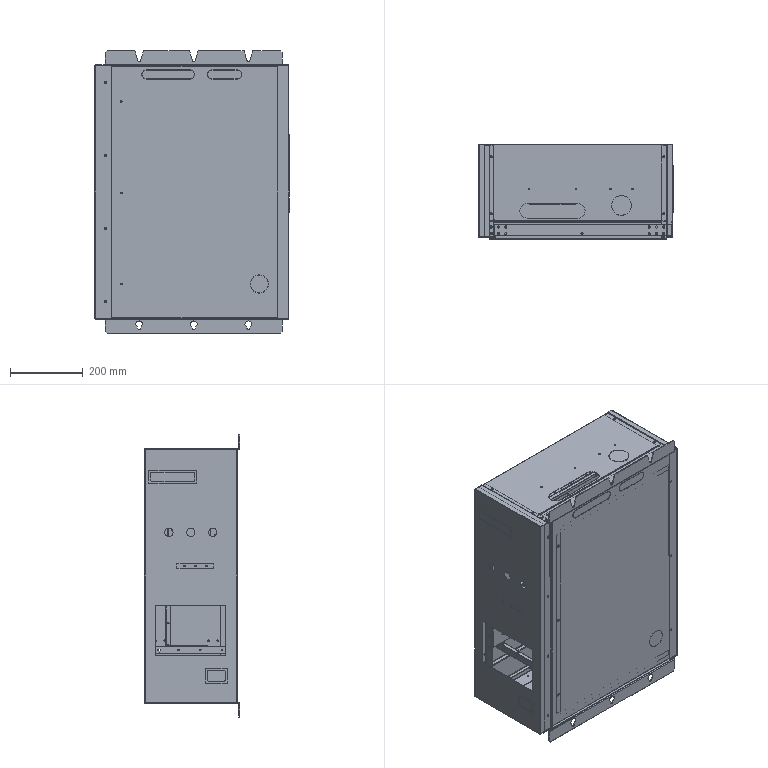Part | SolidWorks | features BaseBody 46 | 46 solids | 3266 faces | volume 3525284 mm3 | cylinder 1863 | plane 1237 | cone 102 | spline 64 | commonest cylinder face diameters 5 x441 6 x240 4 x218 3.3 x138 4.5 x124 8 x114